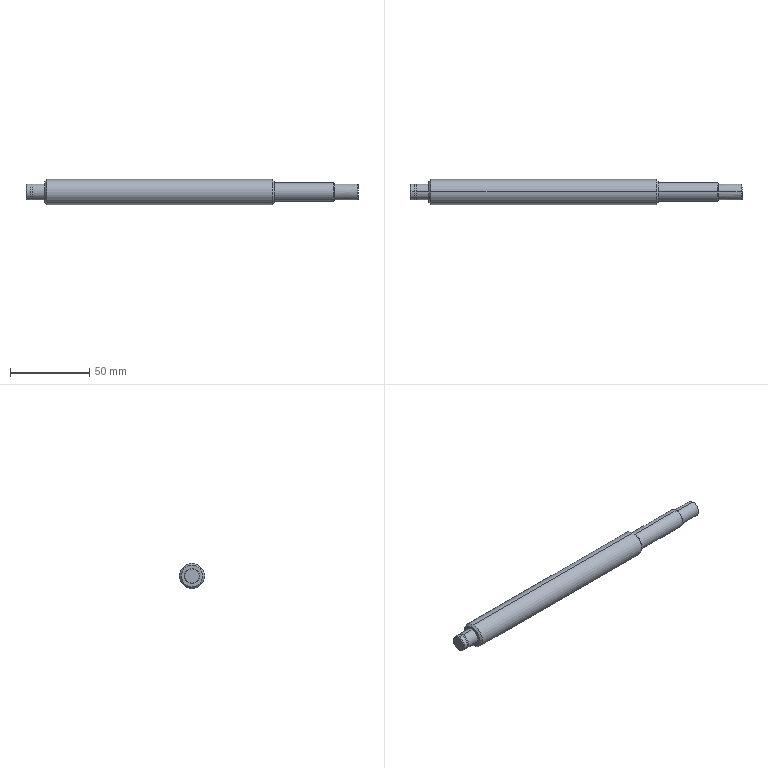Part | SolidWorks | features MoveFace 2, BaseBody 1 | 1 solid | 29 faces | box 210 x 16 x 16 mm | volume 35481 mm3 | cylinder 12 | cone 10 | plane 7 | commonest cylinder face diameters 10 x6 9.6 x2 12 x2 16 x2
STEP:
#1=CARTESIAN_POINT('',(155.773,8.,0.));
#2=VERTEX_POINT('',#1);
#3=CARTESIAN_POINT('',(155.773,0.,-8.));
#4=VERTEX_POINT('',#3);
#5=CARTESIAN_POINT('',(155.773,0.,0.));
#6=DIRECTION('',(-1.,0.,0.));
#7=DIRECTION('',(0.,0.,1.));
#8=AXIS2_PLACEMENT_3D('',#5,#6,#7);
#9=CIRCLE('',#8,8.);
#10=EDGE_CURVE('',#2,#4,#9,.T.);
#11=ORIENTED_EDGE('',*,*,#10,.T.);
#12=CARTESIAN_POINT('',(13.227,0.,-8.));
#13=VERTEX_POINT('',#12);
#14=CARTESIAN_POINT('',(500.,0.,-8.));
#15=DIRECTION('',(-1.,0.,0.));
#16=VECTOR('',#15,1000.);
#17=LINE('',#14,#16);
#18=EDGE_CURVE('',#4,#13,#17,.T.);
#19=ORIENTED_EDGE('',*,*,#18,.T.);
#20=CARTESIAN_POINT('',(13.227,8.,0.));
#21=VERTEX_POINT('',#20);
#22=CARTESIAN_POINT('',(13.227,0.,0.));
#23=DIRECTION('',(1.,0.,0.));
#24=DIRECTION('',(0.,0.,1.));
#25=AXIS2_PLACEMENT_3D('',#22,#23,#24);
#26=CIRCLE('',#25,8.);
#27=EDGE_CURVE('',#13,#21,#26,.T.);
#28=ORIENTED_EDGE('',*,*,#27,.T.);
#29=CARTESIAN_POINT('',(13.227,0.,8.));
#30=VERTEX_POINT('',#29);
#31=CARTESIAN_POINT('',(13.227,0.,0.));
#32=DIRECTION('',(1.,0.,0.));
#33=DIRECTION('',(0.,0.,1.));
#34=AXIS2_PLACEMENT_3D('',#31,#32,#33);
#35=CIRCLE('',#34,8.);
#36=EDGE_CURVE('',#21,#30,#35,.T.);
#37=ORIENTED_EDGE('',*,*,#36,.T.);
#38=CARTESIAN_POINT('',(155.773,0.,8.));
#39=VERTEX_POINT('',#38);
#40=CARTESIAN_POINT('',(500.,0.,8.));
#41=DIRECTION('',(-1.,0.,0.));
#42=VECTOR('',#41,1000.);
#43=LINE('',#40,#42);
#44=EDGE_CURVE('',#39,#30,#43,.T.);
#45=ORIENTED_EDGE('',*,*,#44,.F.);
#46=CARTESIAN_POINT('',(155.773,0.,0.));
#47=DIRECTION('',(-1.,0.,0.));
#48=DIRECTION('',(0.,0.,1.));
#49=AXIS2_PLACEMENT_3D('',#46,#47,#48);
#50=CIRCLE('',#49,8.);
#51=EDGE_CURVE('',#39,#2,#50,.T.);
#52=ORIENTED_EDGE('',*,*,#51,.T.);
#53=EDGE_LOOP('',(#11,#19,#28,#37,#45,#52));
#54=FACE_OUTER_BOUND('',#53,.T.);
#55=CARTESIAN_POINT('',(500.,0.,0.));
#56=DIRECTION('',(-1.,0.,0.));
#57=DIRECTION('',(0.,0.,1.));
#58=AXIS2_PLACEMENT_3D('',#55,#56,#57);
#59=CYLINDRICAL_SURFACE('',#58,8.);
#60=ADVANCED_FACE('',(#54),#59,.T.);
#61=CARTESIAN_POINT('',(12.,6.773,0.));
#62=VERTEX_POINT('',#61);
#63=CARTESIAN_POINT('',(12.,-6.773,0.));
#64=VERTEX_POINT('',#63);
#65=CARTESIAN_POINT('',(12.,0.,0.));
#66=DIRECTION('',(1.,0.,0.));
#67=DIRECTION('',(0.,1.,0.));
#68=AXIS2_PLACEMENT_3D('',#65,#66,#67);
#69=CIRCLE('',#68,6.773);
#70=EDGE_CURVE('',#62,#64,#69,.T.);
#71=ORIENTED_EDGE('',*,*,#70,.T.);
#72=CARTESIAN_POINT('',(13.227,-8.,0.));
#73=VERTEX_POINT('',#72);
#74=CARTESIAN_POINT('',(13.227,-8.,0.));
#75=DIRECTION('',(0.7071,-0.7071,0.));
#76=VECTOR('',#75,1000.);
#77=LINE('',#74,#76);
#78=EDGE_CURVE('',#64,#73,#77,.T.);
#79=ORIENTED_EDGE('',*,*,#78,.T.);
#80=CARTESIAN_POINT('',(13.227,0.,0.));
#81=DIRECTION('',(1.,0.,0.));
#82=DIRECTION('',(0.,0.,1.));
#83=AXIS2_PLACEMENT_3D('',#80,#81,#82);
#84=CIRCLE('',#83,8.);
#85=EDGE_CURVE('',#30,#73,#84,.T.);
#86=ORIENTED_EDGE('',*,*,#85,.F.);
#87=ORIENTED_EDGE('',*,*,#36,.F.);
#88=CARTESIAN_POINT('',(13.227,8.,0.));
#89=DIRECTION('',(0.7071,0.7071,0.));
#90=VECTOR('',#89,1000.);
#91=LINE('',#88,#90);
#92=EDGE_CURVE('',#62,#21,#91,.T.);
#93=ORIENTED_EDGE('',*,*,#92,.F.);
#94=EDGE_LOOP('',(#71,#79,#86,#87,#93));
#95=FACE_OUTER_BOUND('',#94,.T.);
#96=CARTESIAN_POINT('',(13.227,0.,0.));
#97=DIRECTION('',(1.,0.,0.));
#98=DIRECTION('',(0.,1.,0.));
#99=AXIS2_PLACEMENT_3D('',#96,#97,#98);
#100=CONICAL_SURFACE('',#99,8.,0.7854);
#101=ADVANCED_FACE('',(#95),#100,.T.);
#102=CARTESIAN_POINT('',(157.,-6.773,0.));
#103=VERTEX_POINT('',#102);
#104=CARTESIAN_POINT('',(157.,6.773,0.));
#105=VERTEX_POINT('',#104);
#106=CARTESIAN_POINT('',(157.,0.,0.));
#107=DIRECTION('',(-1.,0.,0.));
#108=DIRECTION('',(0.,-1.,0.));
#109=AXIS2_PLACEMENT_3D('',#106,#107,#108);
#110=CIRCLE('',#109,6.773);
#111=EDGE_CURVE('',#103,#105,#110,.T.);
#112=ORIENTED_EDGE('',*,*,#111,.T.);
#113=CARTESIAN_POINT('',(155.773,8.,0.));
#114=DIRECTION('',(-0.7071,0.7071,0.));
#115=VECTOR('',#114,1000.);
#116=LINE('',#113,#115);
#117=EDGE_CURVE('',#105,#2,#116,.T.);
#118=ORIENTED_EDGE('',*,*,#117,.T.);
#119=ORIENTED_EDGE('',*,*,#51,.F.);
#120=CARTESIAN_POINT('',(155.773,-8.,0.));
#121=VERTEX_POINT('',#120);
#122=CARTESIAN_POINT('',(155.773,0.,0.));
#123=DIRECTION('',(-1.,0.,0.));
#124=DIRECTION('',(0.,0.,1.));
#125=AXIS2_PLACEMENT_3D('',#122,#123,#124);
#126=CIRCLE('',#125,8.);
#127=EDGE_CURVE('',#121,#39,#126,.T.);
#128=ORIENTED_EDGE('',*,*,#127,.F.);
#129=CARTESIAN_POINT('',(155.773,-8.,0.));
#130=DIRECTION('',(-0.7071,-0.7071,0.));
#131=VECTOR('',#130,1000.);
#132=LINE('',#129,#131);
#133=EDGE_CURVE('',#103,#121,#132,.T.);
#134=ORIENTED_EDGE('',*,*,#133,.F.);
#135=EDGE_LOOP('',(#112,#118,#119,#128,#134));
#136=FACE_OUTER_BOUND('',#135,.T.);
#137=CARTESIAN_POINT('',(155.773,0.,0.));
#138=DIRECTION('',(-1.,0.,0.));
#139=DIRECTION('',(0.,-1.,0.));
#140=AXIS2_PLACEMENT_3D('',#137,#138,#139);
#141=CONICAL_SURFACE('',#140,8.,0.7854);
#142=ADVANCED_FACE('',(#136),#141,.T.);
#143=CARTESIAN_POINT('',(12.,0.,5.));
#144=VERTEX_POINT('',#143);
#145=CARTESIAN_POINT('',(12.,0.,-5.));
#146=VERTEX_POINT('',#145);
#147=CARTESIAN_POINT('',(12.,0.,0.));
#148=DIRECTION('',(-1.,0.,0.));
#149=DIRECTION('',(0.,0.,1.));
#150=AXIS2_PLACEMENT_3D('',#147,#148,#149);
#151=CIRCLE('',#150,5.);
#152=EDGE_CURVE('',#144,#146,#151,.T.);
#153=ORIENTED_EDGE('',*,*,#152,.T.);
#154=CARTESIAN_POINT('',(4.,0.,-5.));
#155=VERTEX_POINT('',#154);
#156=CARTESIAN_POINT('',(500.,0.,-5.));
#157=DIRECTION('',(-1.,0.,0.));
#158=VECTOR('',#157,1000.);
#159=LINE('',#156,#158);
#160=EDGE_CURVE('',#146,#155,#159,.T.);
#161=ORIENTED_EDGE('',*,*,#160,.T.);
#162=CARTESIAN_POINT('',(4.,0.,5.));
#163=VERTEX_POINT('',#162);
#164=CARTESIAN_POINT('',(4.,0.,0.));
#165=DIRECTION('',(1.,0.,0.));
#166=DIRECTION('',(0.,0.,1.));
#167=AXIS2_PLACEMENT_3D('',#164,#165,#166);
#168=CIRCLE('',#167,5.);
#169=EDGE_CURVE('',#155,#163,#168,.T.);
#170=ORIENTED_EDGE('',*,*,#169,.T.);
#171=CARTESIAN_POINT('',(500.,0.,5.));
#172=DIRECTION('',(-1.,0.,0.));
#173=VECTOR('',#172,1000.);
#174=LINE('',#171,#173);
#175=EDGE_CURVE('',#144,#163,#174,.T.);
#176=ORIENTED_EDGE('',*,*,#175,.F.);
#177=EDGE_LOOP('',(#153,#161,#170,#176));
#178=FACE_OUTER_BOUND('',#177,.T.);
#179=CARTESIAN_POINT('',(500.,0.,0.));
#180=DIRECTION('',(-1.,0.,0.));
#181=DIRECTION('',(0.,0.,1.));
#182=AXIS2_PLACEMENT_3D('',#179,#180,#181);
#183=CYLINDRICAL_SURFACE('',#182,5.);
#184=ADVANCED_FACE('',(#178),#183,.T.);
#185=CARTESIAN_POINT('',(194.5,0.,6.));
#186=VERTEX_POINT('',#185);
#187=CARTESIAN_POINT('',(194.5,0.,-6.));
#188=VERTEX_POINT('',#187);
#189=CARTESIAN_POINT('',(194.5,0.,0.));
#190=DIRECTION('',(-1.,0.,0.));
#191=DIRECTION('',(0.,0.,1.));
#192=AXIS2_PLACEMENT_3D('',#189,#190,#191);
#193=CIRCLE('',#192,6.);
#194=EDGE_CURVE('',#186,#188,#193,.T.);
#195=ORIENTED_EDGE('',*,*,#194,.T.);
#196=CARTESIAN_POINT('',(157.,0.,-6.));
#197=VERTEX_POINT('',#196);
#198=CARTESIAN_POINT('',(500.,0.,-6.));
#199=DIRECTION('',(-1.,0.,0.));
#200=VECTOR('',#199,1000.);
#201=LINE('',#198,#200);
#202=EDGE_CURVE('',#188,#197,#201,.T.);
#203=ORIENTED_EDGE('',*,*,#202,.T.);
#204=CARTESIAN_POINT('',(157.,0.,6.));
#205=VERTEX_POINT('',#204);
#206=CARTESIAN_POINT('',(157.,0.,0.));
#207=DIRECTION('',(1.,0.,0.));
#208=DIRECTION('',(0.,0.,1.));
#209=AXIS2_PLACEMENT_3D('',#206,#207,#208);
#210=CIRCLE('',#209,6.);
#211=EDGE_CURVE('',#197,#205,#210,.T.);
#212=ORIENTED_EDGE('',*,*,#211,.T.);
#213=CARTESIAN_POINT('',(500.,0.,6.));
#214=DIRECTION('',(-1.,0.,0.));
#215=VECTOR('',#214,1000.);
#216=LINE('',#213,#215);
#217=EDGE_CURVE('',#186,#205,#216,.T.);
#218=ORIENTED_EDGE('',*,*,#217,.F.);
#219=EDGE_LOOP('',(#195,#203,#212,#218));
#220=FACE_OUTER_BOUND('',#219,.T.);
#221=CARTESIAN_POINT('',(500.,0.,0.));
#222=DIRECTION('',(-1.,0.,0.));
#223=DIRECTION('',(0.,0.,1.));
#224=AXIS2_PLACEMENT_3D('',#221,#222,#223);
#225=CYLINDRICAL_SURFACE('',#224,6.);
#226=ADVANCED_FACE('',(#220),#225,.T.);
#227=CARTESIAN_POINT('',(195.,0.,5.5));
#228=VERTEX_POINT('',#227);
#229=CARTESIAN_POINT('',(195.,0.,-5.5));
#230=VERTEX_POINT('',#229);
#231=CARTESIAN_POINT('',(195.,0.,0.));
#232=DIRECTION('',(-1.,0.,0.));
#233=DIRECTION('',(0.,0.,1.));
#234=AXIS2_PLACEMENT_3D('',#231,#232,#233);
#235=CIRCLE('',#234,5.5);
#236=EDGE_CURVE('',#228,#230,#235,.T.);
#237=ORIENTED_EDGE('',*,*,#236,.T.);
#238=CARTESIAN_POINT('',(194.5,0.,-6.));
#239=DIRECTION('',(-0.7071,0.,-0.7071));
#240=VECTOR('',#239,1000.);
#241=LINE('',#238,#240);
#242=EDGE_CURVE('',#230,#188,#241,.T.);
#243=ORIENTED_EDGE('',*,*,#242,.T.);
#244=ORIENTED_EDGE('',*,*,#194,.F.);
#245=CARTESIAN_POINT('',(194.5,0.,6.));
#246=DIRECTION('',(-0.7071,0.,0.7071));
#247=VECTOR('',#246,1000.);
#248=LINE('',#245,#247);
#249=EDGE_CURVE('',#228,#186,#248,.T.);
#250=ORIENTED_EDGE('',*,*,#249,.F.);
#251=EDGE_LOOP('',(#237,#243,#244,#250));
#252=FACE_OUTER_BOUND('',#251,.T.);
#253=CARTESIAN_POINT('',(194.5,0.,0.));
#254=DIRECTION('',(-1.,0.,0.));
#255=DIRECTION('',(0.,0.,1.));
#256=AXIS2_PLACEMENT_3D('',#253,#254,#255);
#257=CONICAL_SURFACE('',#256,6.,0.7854);
#258=ADVANCED_FACE('',(#252),#257,.T.);
#259=CARTESIAN_POINT('',(4.,0.,4.8));
#260=VERTEX_POINT('',#259);
#261=CARTESIAN_POINT('',(4.,0.,-4.8));
#262=VERTEX_POINT('',#261);
#263=CARTESIAN_POINT('',(4.,0.,0.));
#264=DIRECTION('',(-1.,0.,0.));
#265=DIRECTION('',(0.,0.,1.));
#266=AXIS2_PLACEMENT_3D('',#263,#264,#265);
#267=CIRCLE('',#266,4.8);
#268=EDGE_CURVE('',#260,#262,#267,.T.);
#269=ORIENTED_EDGE('',*,*,#268,.T.);
#270=CARTESIAN_POINT('',(2.85,0.,-4.8));
#271=VERTEX_POINT('',#270);
#272=CARTESIAN_POINT('',(500.,0.,-4.8));
#273=DIRECTION('',(-1.,0.,0.));
#274=VECTOR('',#273,1000.);
#275=LINE('',#272,#274);
#276=EDGE_CURVE('',#262,#271,#275,.T.);
#277=ORIENTED_EDGE('',*,*,#276,.T.);
#278=CARTESIAN_POINT('',(2.85,0.,4.8));
#279=VERTEX_POINT('',#278);
#280=CARTESIAN_POINT('',(2.85,0.,0.));
#281=DIRECTION('',(1.,0.,0.));
#282=DIRECTION('',(0.,0.,1.));
#283=AXIS2_PLACEMENT_3D('',#280,#281,#282);
#284=CIRCLE('',#283,4.8);
#285=EDGE_CURVE('',#271,#279,#284,.T.);
#286=ORIENTED_EDGE('',*,*,#285,.T.);
#287=CARTESIAN_POINT('',(500.,0.,4.8));
#288=DIRECTION('',(-1.,0.,0.));
#289=VECTOR('',#288,1000.);
#290=LINE('',#287,#289);
#291=EDGE_CURVE('',#260,#279,#290,.T.);
#292=ORIENTED_EDGE('',*,*,#291,.F.);
#293=EDGE_LOOP('',(#269,#277,#286,#292));
#294=FACE_OUTER_BOUND('',#293,.T.);
#295=CARTESIAN_POINT('',(500.,0.,0.));
#296=DIRECTION('',(-1.,0.,0.));
#297=DIRECTION('',(0.,0.,1.));
#298=AXIS2_PLACEMENT_3D('',#295,#296,#297);
#299=CYLINDRICAL_SURFACE('',#298,4.8);
#300=ADVANCED_FACE('',(#294),#299,.T.);
#301=CARTESIAN_POINT('',(209.5,5.,0.));
#302=VERTEX_POINT('',#301);
#303=CARTESIAN_POINT('',(209.5,0.,-5.));
#304=VERTEX_POINT('',#303);
#305=CARTESIAN_POINT('',(209.5,0.,0.));
#306=DIRECTION('',(-1.,0.,0.));
#307=DIRECTION('',(0.,0.,1.));
#308=AXIS2_PLACEMENT_3D('',#305,#306,#307);
#309=CIRCLE('',#308,5.);
#310=EDGE_CURVE('',#302,#304,#309,.T.);
#311=ORIENTED_EDGE('',*,*,#310,.T.);
#312=CARTESIAN_POINT('',(195.,0.,-5.));
#313=VERTEX_POINT('',#312);
#314=CARTESIAN_POINT('',(500.,0.,-5.));
#315=DIRECTION('',(-1.,0.,0.));
#316=VECTOR('',#315,1000.);
#317=LINE('',#314,#316);
#318=EDGE_CURVE('',#304,#313,#317,.T.);
#319=ORIENTED_EDGE('',*,*,#318,.T.);
#320=CARTESIAN_POINT('',(195.,0.,5.));
#321=VERTEX_POINT('',#320);
#322=CARTESIAN_POINT('',(195.,0.,0.));
#323=DIRECTION('',(1.,0.,0.));
#324=DIRECTION('',(0.,0.,1.));
#325=AXIS2_PLACEMENT_3D('',#322,#323,#324);
#326=CIRCLE('',#325,5.);
#327=EDGE_CURVE('',#313,#321,#326,.T.);
#328=ORIENTED_EDGE('',*,*,#327,.T.);
#329=CARTESIAN_POINT('',(209.5,0.,5.));
#330=VERTEX_POINT('',#329);
#331=CARTESIAN_POINT('',(500.,0.,5.));
#332=DIRECTION('',(-1.,0.,0.));
#333=VECTOR('',#332,1000.);
#334=LINE('',#331,#333);
#335=EDGE_CURVE('',#330,#321,#334,.T.);
#336=ORIENTED_EDGE('',*,*,#335,.F.);
#337=CARTESIAN_POINT('',(209.5,0.,0.));
#338=DIRECTION('',(-1.,0.,0.));
#339=DIRECTION('',(0.,0.,1.));
#340=AXIS2_PLACEMENT_3D('',#337,#338,#339);
#341=CIRCLE('',#340,5.);
#342=EDGE_CURVE('',#330,#302,#341,.T.);
#343=ORIENTED_EDGE('',*,*,#342,.T.);
#344=EDGE_LOOP('',(#311,#319,#328,#336,#343));
#345=FACE_OUTER_BOUND('',#344,.T.);
#346=CARTESIAN_POINT('',(500.,0.,0.));
#347=DIRECTION('',(-1.,0.,0.));
#348=DIRECTION('',(0.,0.,1.));
#349=AXIS2_PLACEMENT_3D('',#346,#347,#348);
#350=CYLINDRICAL_SURFACE('',#349,5.);
#351=ADVANCED_FACE('',(#345),#350,.T.);
#352=CARTESIAN_POINT('',(2.85,0.,5.));
#353=VERTEX_POINT('',#352);
#354=CARTESIAN_POINT('',(2.85,0.,-5.));
#355=VERTEX_POINT('',#354);
#356=CARTESIAN_POINT('',(2.85,0.,0.));
#357=DIRECTION('',(-1.,0.,0.));
#358=DIRECTION('',(0.,0.,1.));
#359=AXIS2_PLACEMENT_3D('',#356,#357,#358);
#360=CIRCLE('',#359,5.);
#361=EDGE_CURVE('',#353,#355,#360,.T.);
#362=ORIENTED_EDGE('',*,*,#361,.T.);
#363=CARTESIAN_POINT('',(0.5,0.,-5.));
#364=VERTEX_POINT('',#363);
#365=CARTESIAN_POINT('',(500.,0.,-5.));
#366=DIRECTION('',(-1.,0.,0.));
#367=VECTOR('',#366,1000.);
#368=LINE('',#365,#367);
#369=EDGE_CURVE('',#355,#364,#368,.T.);
#370=ORIENTED_EDGE('',*,*,#369,.T.);
#371=CARTESIAN_POINT('',(0.5,0.,5.));
#372=VERTEX_POINT('',#371);
#373=CARTESIAN_POINT('',(0.5,0.,0.));
#374=DIRECTION('',(1.,0.,0.));
#375=DIRECTION('',(0.,0.,1.));
#376=AXIS2_PLACEMENT_3D('',#373,#374,#375);
#377=CIRCLE('',#376,5.);
#378=EDGE_CURVE('',#364,#372,#377,.T.);
#379=ORIENTED_EDGE('',*,*,#378,.T.);
#380=CARTESIAN_POINT('',(500.,0.,5.));
#381=DIRECTION('',(-1.,0.,0.));
#382=VECTOR('',#381,1000.);
#383=LINE('',#380,#382);
#384=EDGE_CURVE('',#353,#372,#383,.T.);
#385=ORIENTED_EDGE('',*,*,#384,.F.);
#386=EDGE_LOOP('',(#362,#370,#379,#385));
#387=FACE_OUTER_BOUND('',#386,.T.);
#388=CARTESIAN_POINT('',(500.,0.,0.));
#389=DIRECTION('',(-1.,0.,0.));
#390=DIRECTION('',(0.,0.,1.));
#391=AXIS2_PLACEMENT_3D('',#388,#389,#390);
#392=CYLINDRICAL_SURFACE('',#391,5.);
#393=ADVANCED_FACE('',(#387),#392,.T.);
#394=CARTESIAN_POINT('',(210.,-4.5,0.));
#395=VERTEX_POINT('',#394);
#396=CARTESIAN_POINT('',(210.,4.5,0.));
#397=VERTEX_POINT('',#396);
#398=CARTESIAN_POINT('',(210.,0.,0.));
#399=DIRECTION('',(-1.,0.,0.));
#400=DIRECTION('',(0.,-1.,0.));
#401=AXIS2_PLACEMENT_3D('',#398,#399,#400);
#402=CIRCLE('',#401,4.5);
#403=EDGE_CURVE('',#395,#397,#402,.T.);
#404=ORIENTED_EDGE('',*,*,#403,.T.);
#405=CARTESIAN_POINT('',(209.5,5.,0.));
#406=DIRECTION('',(-0.7071,0.7071,0.));
#407=VECTOR('',#406,1000.);
#408=LINE('',#405,#407);
#409=EDGE_CURVE('',#397,#302,#408,.T.);
#410=ORIENTED_EDGE('',*,*,#409,.T.);
#411=ORIENTED_EDGE('',*,*,#342,.F.);
#412=CARTESIAN_POINT('',(209.5,-5.,0.));
#413=VERTEX_POINT('',#412);
#414=CARTESIAN_POINT('',(209.5,0.,0.));
#415=DIRECTION('',(-1.,0.,0.));
#416=DIRECTION('',(0.,0.,1.));
#417=AXIS2_PLACEMENT_3D('',#414,#415,#416);
#418=CIRCLE('',#417,5.);
#419=EDGE_CURVE('',#413,#330,#418,.T.);
#420=ORIENTED_EDGE('',*,*,#419,.F.);
#421=CARTESIAN_POINT('',(209.5,-5.,0.));
#422=DIRECTION('',(-0.7071,-0.7071,0.));
#423=VECTOR('',#422,1000.);
#424=LINE('',#421,#423);
#425=EDGE_CURVE('',#395,#413,#424,.T.);
#426=ORIENTED_EDGE('',*,*,#425,.F.);
#427=EDGE_LOOP('',(#404,#410,#411,#420,#426));
#428=FACE_OUTER_BOUND('',#427,.T.);
#429=CARTESIAN_POINT('',(209.5,0.,0.));
#430=DIRECTION('',(-1.,0.,0.));
#431=DIRECTION('',(0.,-1.,0.));
#432=AXIS2_PLACEMENT_3D('',#429,#430,#431);
#433=CONICAL_SURFACE('',#432,5.,0.7854);
#434=ADVANCED_FACE('',(#428),#433,.T.);
#435=CARTESIAN_POINT('',(0.,0.,-4.5));
#436=VERTEX_POINT('',#435);
#437=CARTESIAN_POINT('',(0.,0.,4.5));
#438=VERTEX_POINT('',#437);
#439=CARTESIAN_POINT('',(0.,0.,0.));
#440=DIRECTION('',(1.,0.,0.));
#441=DIRECTION('',(0.,0.,-1.));
#442=AXIS2_PLACEMENT_3D('',#439,#440,#441);
#443=CIRCLE('',#442,4.5);
#444=EDGE_CURVE('',#436,#438,#443,.T.);
#445=ORIENTED_EDGE('',*,*,#444,.T.);
#446=CARTESIAN_POINT('',(0.5,0.,5.));
#447=DIRECTION('',(0.7071,0.,0.7071));
#448=VECTOR('',#447,1000.);
#449=LINE('',#446,#448);
#450=EDGE_CURVE('',#438,#372,#449,.T.);
#451=ORIENTED_EDGE('',*,*,#450,.T.);
#452=ORIENTED_EDGE('',*,*,#378,.F.);
#453=CARTESIAN_POINT('',(0.5,0.,-5.));
#454=DIRECTION('',(0.7071,0.,-0.7071));
#455=VECTOR('',#454,1000.);
#456=LINE('',#453,#455);
#457=EDGE_CURVE('',#436,#364,#456,.T.);
#458=ORIENTED_EDGE('',*,*,#457,.F.);
#459=EDGE_LOOP('',(#445,#451,#452,#458));
#460=FACE_OUTER_BOUND('',#459,.T.);
#461=CARTESIAN_POINT('',(0.5,0.,0.));
#462=DIRECTION('',(1.,0.,0.));
#463=DIRECTION('',(0.,0.,-1.));
#464=AXIS2_PLACEMENT_3D('',#461,#462,#463);
#465=CONICAL_SURFACE('',#464,5.,0.7854);
#466=ADVANCED_FACE('',(#460),#465,.T.);
#467=ORIENTED_EDGE('',*,*,#18,.F.);
#468=CARTESIAN_POINT('',(155.773,0.,0.));
#469=DIRECTION('',(-1.,0.,0.));
#470=DIRECTION('',(0.,0.,1.));
#471=AXIS2_PLACEMENT_3D('',#468,#469,#470);
#472=CIRCLE('',#471,8.);
#473=EDGE_CURVE('',#4,#121,#472,.T.);
#474=ORIENTED_EDGE('',*,*,#473,.T.);
#475=ORIENTED_EDGE('',*,*,#127,.T.);
#476=ORIENTED_EDGE('',*,*,#44,.T.);
#477=ORIENTED_EDGE('',*,*,#85,.T.);
#478=CARTESIAN_POINT('',(13.227,0.,0.));
#479=DIRECTION('',(1.,0.,0.));
#480=DIRECTION('',(0.,0.,1.));
#481=AXIS2_PLACEMENT_3D('',#478,#479,#480);
#482=CIRCLE('',#481,8.);
#483=EDGE_CURVE('',#73,#13,#482,.T.);
#484=ORIENTED_EDGE('',*,*,#483,.T.);
#485=EDGE_LOOP('',(#467,#474,#475,#476,#477,#484));
#486=FACE_OUTER_BOUND('',#485,.T.);
#487=CARTESIAN_POINT('',(500.,0.,0.));
#488=DIRECTION('',(-1.,0.,0.));
#489=DIRECTION('',(0.,0.,1.));
#490=AXIS2_PLACEMENT_3D('',#487,#488,#489);
#491=CYLINDRICAL_SURFACE('',#490,8.);
#492=ADVANCED_FACE('',(#486),#491,.T.);
#493=ORIENTED_EDGE('',*,*,#78,.F.);
#494=CARTESIAN_POINT('',(12.,0.,0.));
#495=DIRECTION('',(1.,0.,0.));
#496=DIRECTION('',(0.,1.,0.));
#497=AXIS2_PLACEMENT_3D('',#494,#495,#496);
#498=CIRCLE('',#497,6.773);
#499=EDGE_CURVE('',#64,#62,#498,.T.);
#500=ORIENTED_EDGE('',*,*,#499,.T.);
#501=ORIENTED_EDGE('',*,*,#92,.T.);
#502=ORIENTED_EDGE('',*,*,#27,.F.);
#503=ORIENTED_EDGE('',*,*,#483,.F.);
#504=EDGE_LOOP('',(#493,#500,#501,#502,#503));
#505=FACE_OUTER_BOUND('',#504,.T.);
#506=CARTESIAN_POINT('',(13.227,0.,0.));
#507=DIRECTION('',(1.,0.,0.));
#508=DIRECTION('',(0.,1.,0.));
#509=AXIS2_PLACEMENT_3D('',#506,#507,#508);
#510=CONICAL_SURFACE('',#509,8.,0.7854);
#511=ADVANCED_FACE('',(#505),#510,.T.);
#512=ORIENTED_EDGE('',*,*,#117,.F.);
#513=CARTESIAN_POINT('',(157.,0.,0.));
#514=DIRECTION('',(-1.,0.,0.));
#515=DIRECTION('',(0.,-1.,0.));
#516=AXIS2_PLACEMENT_3D('',#513,#514,#515);
#517=CIRCLE('',#516,6.773);
#518=EDGE_CURVE('',#105,#103,#517,.T.);
#519=ORIENTED_EDGE('',*,*,#518,.T.);
#520=ORIENTED_EDGE('',*,*,#133,.T.);
#521=ORIENTED_EDGE('',*,*,#473,.F.);
#522=ORIENTED_EDGE('',*,*,#10,.F.);
#523=EDGE_LOOP('',(#512,#519,#520,#521,#522));
#524=FACE_OUTER_BOUND('',#523,.T.);
#525=CARTESIAN_POINT('',(155.773,0.,0.));
#526=DIRECTION('',(-1.,0.,0.));
#527=DIRECTION('',(0.,-1.,0.));
#528=AXIS2_PLACEMENT_3D('',#525,#526,#527);
#529=CONICAL_SURFACE('',#528,8.,0.7854);
#530=ADVANCED_FACE('',(#524),#529,.T.);
#531=ORIENTED_EDGE('',*,*,#152,.F.);
#532=CARTESIAN_POINT('',(12.,0.,0.));
#533=DIRECTION('',(-1.,0.,0.));
#534=DIRECTION('',(0.,0.,1.));
#535=AXIS2_PLACEMENT_3D('',#532,#533,#534);
#536=CIRCLE('',#535,5.);
#537=EDGE_CURVE('',#146,#144,#536,.T.);
#538=ORIENTED_EDGE('',*,*,#537,.F.);
#539=EDGE_LOOP('',(#531,#538));
#540=FACE_BOUND('',#539,.T.);
#541=ORIENTED_EDGE('',*,*,#70,.F.);
#542=ORIENTED_EDGE('',*,*,#499,.F.);
#543=EDGE_LOOP('',(#541,#542));
#544=FACE_OUTER_BOUND('',#543,.T.);
#545=CARTESIAN_POINT('',(12.,5.,0.));
#546=DIRECTION('',(1.,0.,0.));
#547=DIRECTION('',(0.,0.,-1.));
#548=AXIS2_PLACEMENT_3D('',#545,#546,#547);
#549=PLANE('',#548);
#550=ADVANCED_FACE('',(#540,#544),#549,.F.);
#551=ORIENTED_EDGE('',*,*,#111,.F.);
#552=ORIENTED_EDGE('',*,*,#518,.F.);
#553=EDGE_LOOP('',(#551,#552));
#554=FACE_OUTER_BOUND('',#553,.T.);
#555=CARTESIAN_POINT('',(157.,0.,0.));
#556=DIRECTION('',(1.,0.,0.));
#557=DIRECTION('',(0.,0.,1.));
#558=AXIS2_PLACEMENT_3D('',#555,#556,#557);
#559=CIRCLE('',#558,6.);
#560=EDGE_CURVE('',#205,#197,#559,.T.);
#561=ORIENTED_EDGE('',*,*,#560,.F.);
#562=ORIENTED_EDGE('',*,*,#211,.F.);
#563=EDGE_LOOP('',(#561,#562));
#564=FACE_BOUND('',#563,.T.);
#565=CARTESIAN_POINT('',(157.,6.773,0.));
#566=DIRECTION('',(-1.,0.,0.));
#567=DIRECTION('',(0.,0.,1.));
#568=AXIS2_PLACEMENT_3D('',#565,#566,#567);
#569=PLANE('',#568);
#570=ADVANCED_FACE('',(#554,#564),#569,.F.);
#571=ORIENTED_EDGE('',*,*,#160,.F.);
#572=ORIENTED_EDGE('',*,*,#537,.T.);
#573=ORIENTED_EDGE('',*,*,#175,.T.);
#574=CARTESIAN_POINT('',(4.,0.,0.));
#575=DIRECTION('',(1.,0.,0.));
#576=DIRECTION('',(0.,0.,1.));
#577=AXIS2_PLACEMENT_3D('',#574,#575,#576);
#578=CIRCLE('',#577,5.);
#579=EDGE_CURVE('',#163,#155,#578,.T.);
#580=ORIENTED_EDGE('',*,*,#579,.T.);
#581=EDGE_LOOP('',(#571,#572,#573,#580));
#582=FACE_OUTER_BOUND('',#581,.T.);
#583=CARTESIAN_POINT('',(500.,0.,0.));
#584=DIRECTION('',(-1.,0.,0.));
#585=DIRECTION('',(0.,0.,1.));
#586=AXIS2_PLACEMENT_3D('',#583,#584,#585);
#587=CYLINDRICAL_SURFACE('',#586,5.);
#588=ADVANCED_FACE('',(#582),#587,.T.);
#589=ORIENTED_EDGE('',*,*,#202,.F.);
#590=CARTESIAN_POINT('',(194.5,0.,0.));
#591=DIRECTION('',(-1.,0.,0.));
#592=DIRECTION('',(0.,0.,1.));
#593=AXIS2_PLACEMENT_3D('',#590,#591,#592);
#594=CIRCLE('',#593,6.);
#595=EDGE_CURVE('',#188,#186,#594,.T.);
#596=ORIENTED_EDGE('',*,*,#595,.T.);
#597=ORIENTED_EDGE('',*,*,#217,.T.);
#598=ORIENTED_EDGE('',*,*,#560,.T.);
#599=EDGE_LOOP('',(#589,#596,#597,#598));
#600=FACE_OUTER_BOUND('',#599,.T.);
#601=CARTESIAN_POINT('',(500.,0.,0.));
#602=DIRECTION('',(-1.,0.,0.));
#603=DIRECTION('',(0.,0.,1.));
#604=AXIS2_PLACEMENT_3D('',#601,#602,#603);
#605=CYLINDRICAL_SURFACE('',#604,6.);
#606=ADVANCED_FACE('',(#600),#605,.T.);
#607=ORIENTED_EDGE('',*,*,#268,.F.);
#608=CARTESIAN_POINT('',(4.,0.,0.));
#609=DIRECTION('',(-1.,0.,0.));
#610=DIRECTION('',(0.,0.,1.));
#611=AXIS2_PLACEMENT_3D('',#608,#609,#610);
#612=CIRCLE('',#611,4.8);
#613=EDGE_CURVE('',#262,#260,#612,.T.);
#614=ORIENTED_EDGE('',*,*,#613,.F.);
#615=EDGE_LOOP('',(#607,#614));
#616=FACE_BOUND('',#615,.T.);
#617=ORIENTED_EDGE('',*,*,#579,.F.);
#618=ORIENTED_EDGE('',*,*,#169,.F.);
#619=EDGE_LOOP('',(#617,#618));
#620=FACE_OUTER_BOUND('',#619,.T.);
#621=CARTESIAN_POINT('',(4.,4.8,0.));
#622=DIRECTION('',(1.,0.,0.));
#623=DIRECTION('',(0.,0.,-1.));
#624=AXIS2_PLACEMENT_3D('',#621,#622,#623);
#625=PLANE('',#624);
#626=ADVANCED_FACE('',(#616,#620),#625,.F.);
#627=ORIENTED_EDGE('',*,*,#242,.F.);
#628=CARTESIAN_POINT('',(195.,0.,0.));
#629=DIRECTION('',(-1.,0.,0.));
#630=DIRECTION('',(0.,0.,1.));
#631=AXIS2_PLACEMENT_3D('',#628,#629,#630);
#632=CIRCLE('',#631,5.5);
#633=EDGE_CURVE('',#230,#228,#632,.T.);
#634=ORIENTED_EDGE('',*,*,#633,.T.);
#635=ORIENTED_EDGE('',*,*,#249,.T.);
#636=ORIENTED_EDGE('',*,*,#595,.F.);
#637=EDGE_LOOP('',(#627,#634,#635,#636));
#638=FACE_OUTER_BOUND('',#637,.T.);
#639=CARTESIAN_POINT('',(194.5,0.,0.));
#640=DIRECTION('',(-1.,0.,0.));
#641=DIRECTION('',(0.,0.,1.));
#642=AXIS2_PLACEMENT_3D('',#639,#640,#641);
#643=CONICAL_SURFACE('',#642,6.,0.7854);
#644=ADVANCED_FACE('',(#638),#643,.T.);
#645=ORIENTED_EDGE('',*,*,#276,.F.);
#646=ORIENTED_EDGE('',*,*,#613,.T.);
#647=ORIENTED_EDGE('',*,*,#291,.T.);
#648=CARTESIAN_POINT('',(2.85,0.,0.));
#649=DIRECTION('',(1.,0.,0.));
#650=DIRECTION('',(0.,0.,1.));
#651=AXIS2_PLACEMENT_3D('',#648,#649,#650);
#652=CIRCLE('',#651,4.8);
#653=EDGE_CURVE('',#279,#271,#652,.T.);
#654=ORIENTED_EDGE('',*,*,#653,.T.);
#655=EDGE_LOOP('',(#645,#646,#647,#654));
#656=FACE_OUTER_BOUND('',#655,.T.);
#657=CARTESIAN_POINT('',(500.,0.,0.));
#658=DIRECTION('',(-1.,0.,0.));
#659=DIRECTION('',(0.,0.,1.));
#660=AXIS2_PLACEMENT_3D('',#657,#658,#659);
#661=CYLINDRICAL_SURFACE('',#660,4.8);
#662=ADVANCED_FACE('',(#656),#661,.T.);
#663=ORIENTED_EDGE('',*,*,#236,.F.);
#664=ORIENTED_EDGE('',*,*,#633,.F.);
#665=EDGE_LOOP('',(#663,#664));
#666=FACE_OUTER_BOUND('',#665,.T.);
#667=CARTESIAN_POINT('',(195.,0.,0.));
#668=DIRECTION('',(1.,0.,0.));
#669=DIRECTION('',(0.,0.,1.));
#670=AXIS2_PLACEMENT_3D('',#667,#668,#669);
#671=CIRCLE('',#670,5.);
#672=EDGE_CURVE('',#321,#313,#671,.T.);
#673=ORIENTED_EDGE('',*,*,#672,.F.);
#674=ORIENTED_EDGE('',*,*,#327,.F.);
#675=EDGE_LOOP('',(#673,#674));
#676=FACE_BOUND('',#675,.T.);
#677=CARTESIAN_POINT('',(195.,5.5,0.));
#678=DIRECTION('',(-1.,0.,0.));
#679=DIRECTION('',(0.,0.,1.));
#680=AXIS2_PLACEMENT_3D('',#677,#678,#679);
#681=PLANE('',#680);
#682=ADVANCED_FACE('',(#666,#676),#681,.F.);
#683=ORIENTED_EDGE('',*,*,#361,.F.);
#684=CARTESIAN_POINT('',(2.85,0.,0.));
#685=DIRECTION('',(-1.,0.,0.));
#686=DIRECTION('',(0.,0.,1.));
#687=AXIS2_PLACEMENT_3D('',#684,#685,#686);
#688=CIRCLE('',#687,5.);
#689=EDGE_CURVE('',#355,#353,#688,.T.);
#690=ORIENTED_EDGE('',*,*,#689,.F.);
#691=EDGE_LOOP('',(#683,#690));
#692=FACE_OUTER_BOUND('',#691,.T.);
#693=ORIENTED_EDGE('',*,*,#653,.F.);
#694=ORIENTED_EDGE('',*,*,#285,.F.);
#695=EDGE_LOOP('',(#693,#694));
#696=FACE_BOUND('',#695,.T.);
#697=CARTESIAN_POINT('',(2.85,5.,0.));
#698=DIRECTION('',(-1.,0.,0.));
#699=DIRECTION('',(0.,0.,1.));
#700=AXIS2_PLACEMENT_3D('',#697,#698,#699);
#701=PLANE('',#700);
#702=ADVANCED_FACE('',(#692,#696),#701,.F.);
#703=ORIENTED_EDGE('',*,*,#318,.F.);
#704=CARTESIAN_POINT('',(209.5,0.,0.));
#705=DIRECTION('',(-1.,0.,0.));
#706=DIRECTION('',(0.,0.,1.));
#707=AXIS2_PLACEMENT_3D('',#704,#705,#706);
#708=CIRCLE('',#707,5.);
#709=EDGE_CURVE('',#304,#413,#708,.T.);
#710=ORIENTED_EDGE('',*,*,#709,.T.);
#711=ORIENTED_EDGE('',*,*,#419,.T.);
#712=ORIENTED_EDGE('',*,*,#335,.T.);
#713=ORIENTED_EDGE('',*,*,#672,.T.);
#714=EDGE_LOOP('',(#703,#710,#711,#712,#713));
#715=FACE_OUTER_BOUND('',#714,.T.);
#716=CARTESIAN_POINT('',(500.,0.,0.));
#717=DIRECTION('',(-1.,0.,0.));
#718=DIRECTION('',(0.,0.,1.));
#719=AXIS2_PLACEMENT_3D('',#716,#717,#718);
#720=CYLINDRICAL_SURFACE('',#719,5.);
#721=ADVANCED_FACE('',(#715),#720,.T.);
#722=ORIENTED_EDGE('',*,*,#369,.F.);
#723=ORIENTED_EDGE('',*,*,#689,.T.);
#724=ORIENTED_EDGE('',*,*,#384,.T.);
#725=CARTESIAN_POINT('',(0.5,0.,0.));
#726=DIRECTION('',(1.,0.,0.));
#727=DIRECTION('',(0.,0.,1.));
#728=AXIS2_PLACEMENT_3D('',#725,#726,#727);
#729=CIRCLE('',#728,5.);
#730=EDGE_CURVE('',#372,#364,#729,.T.);
#731=ORIENTED_EDGE('',*,*,#730,.T.);
#732=EDGE_LOOP('',(#722,#723,#724,#731));
#733=FACE_OUTER_BOUND('',#732,.T.);
#734=CARTESIAN_POINT('',(500.,0.,0.));
#735=DIRECTION('',(-1.,0.,0.));
#736=DIRECTION('',(0.,0.,1.));
#737=AXIS2_PLACEMENT_3D('',#734,#735,#736);
#738=CYLINDRICAL_SURFACE('',#737,5.);
#739=ADVANCED_FACE('',(#733),#738,.T.);
#740=ORIENTED_EDGE('',*,*,#409,.F.);
#741=CARTESIAN_POINT('',(210.,0.,0.));
#742=DIRECTION('',(-1.,0.,0.));
#743=DIRECTION('',(0.,-1.,0.));
#744=AXIS2_PLACEMENT_3D('',#741,#742,#743);
#745=CIRCLE('',#744,4.5);
#746=EDGE_CURVE('',#397,#395,#745,.T.);
#747=ORIENTED_EDGE('',*,*,#746,.T.);
#748=ORIENTED_EDGE('',*,*,#425,.T.);
#749=ORIENTED_EDGE('',*,*,#709,.F.);
#750=ORIENTED_EDGE('',*,*,#310,.F.);
#751=EDGE_LOOP('',(#740,#747,#748,#749,#750));
#752=FACE_OUTER_BOUND('',#751,.T.);
#753=CARTESIAN_POINT('',(209.5,0.,0.));
#754=DIRECTION('',(-1.,0.,0.));
#755=DIRECTION('',(0.,-1.,0.));
#756=AXIS2_PLACEMENT_3D('',#753,#754,#755);
#757=CONICAL_SURFACE('',#756,5.,0.7854);
#758=ADVANCED_FACE('',(#752),#757,.T.);
#759=ORIENTED_EDGE('',*,*,#450,.F.);
#760=CARTESIAN_POINT('',(0.,0.,0.));
#761=DIRECTION('',(1.,0.,0.));
#762=DIRECTION('',(0.,0.,-1.));
#763=AXIS2_PLACEMENT_3D('',#760,#761,#762);
#764=CIRCLE('',#763,4.5);
#765=EDGE_CURVE('',#438,#436,#764,.T.);
#766=ORIENTED_EDGE('',*,*,#765,.T.);
#767=ORIENTED_EDGE('',*,*,#457,.T.);
#768=ORIENTED_EDGE('',*,*,#730,.F.);
#769=EDGE_LOOP('',(#759,#766,#767,#768));
#770=FACE_OUTER_BOUND('',#769,.T.);
#771=CARTESIAN_POINT('',(0.5,0.,0.));
#772=DIRECTION('',(1.,0.,0.));
#773=DIRECTION('',(0.,0.,-1.));
#774=AXIS2_PLACEMENT_3D('',#771,#772,#773);
#775=CONICAL_SURFACE('',#774,5.,0.7854);
#776=ADVANCED_FACE('',(#770),#775,.T.);
#777=ORIENTED_EDGE('',*,*,#403,.F.);
#778=ORIENTED_EDGE('',*,*,#746,.F.);
#779=EDGE_LOOP('',(#777,#778));
#780=FACE_OUTER_BOUND('',#779,.T.);
#781=CARTESIAN_POINT('',(210.,4.5,0.));
#782=DIRECTION('',(-1.,0.,0.));
#783=DIRECTION('',(0.,0.,1.));
#784=AXIS2_PLACEMENT_3D('',#781,#782,#783);
#785=PLANE('',#784);
#786=ADVANCED_FACE('',(#780),#785,.F.);
#787=ORIENTED_EDGE('',*,*,#444,.F.);
#788=ORIENTED_EDGE('',*,*,#765,.F.);
#789=EDGE_LOOP('',(#787,#788));
#790=FACE_OUTER_BOUND('',#789,.T.);
#791=CARTESIAN_POINT('',(0.,0.,0.));
#792=DIRECTION('',(1.,0.,0.));
#793=DIRECTION('',(0.,0.,-1.));
#794=AXIS2_PLACEMENT_3D('',#791,#792,#793);
#795=PLANE('',#794);
#796=ADVANCED_FACE('',(#790),#795,.F.);
#797=CLOSED_SHELL('',(#60,#101,#142,#184,#226,#258,#300,#351,#393,#434,#466,#492,#511,#530,#550,#570,#588,#606,#626,#644,#662,#682,#702,#721,#739,#758,#776,#786,#796));
#798=MANIFOLD_SOLID_BREP('',#797);
#799=CARTESIAN_POINT('',(0.,0.,0.));
#800=DIRECTION('',(0.,0.,1.));
#801=DIRECTION('',(1.,0.,0.));
#802=AXIS2_PLACEMENT_3D('',#799,#800,#801);
#803=(LENGTH_UNIT()NAMED_UNIT(*)SI_UNIT(.MILLI.,.METRE.));
#804=UNCERTAINTY_MEASURE_WITH_UNIT(LENGTH_MEASURE(0.00001),#803,'','');
#805=(NAMED_UNIT(*)PLANE_ANGLE_UNIT()SI_UNIT($,.RADIAN.));
#806=(NAMED_UNIT(*)SI_UNIT($,.STERADIAN.)SOLID_ANGLE_UNIT());
#807=(GEOMETRIC_REPRESENTATION_CONTEXT(3)GLOBAL_UNCERTAINTY_ASSIGNED_CONTEXT((#804))GLOBAL_UNIT_ASSIGNED_CONTEXT((#803,#805,#806))REPRESENTATION_CONTEXT('',''));
#808=ADVANCED_BREP_SHAPE_REPRESENTATION('',(#798,#802),#807);